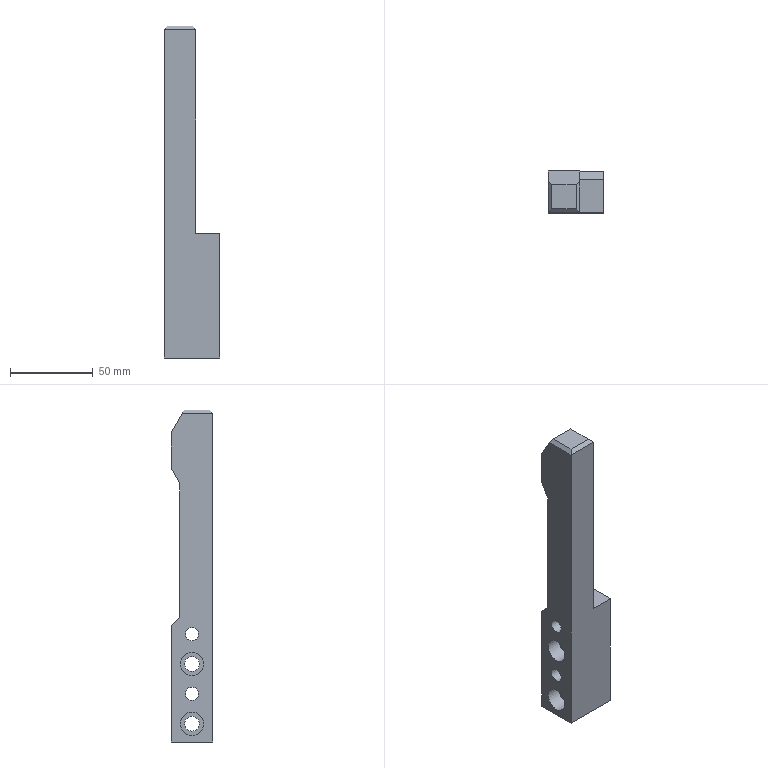Part | STEP file | solid 130 | 1 solid | 24 faces | box 33.5 x 25 x 200.006 mm | volume 103265 mm3 | plane 18 | cylinder 6 | commonest cylinder face diameters 8 x2 9 x2 14 x2